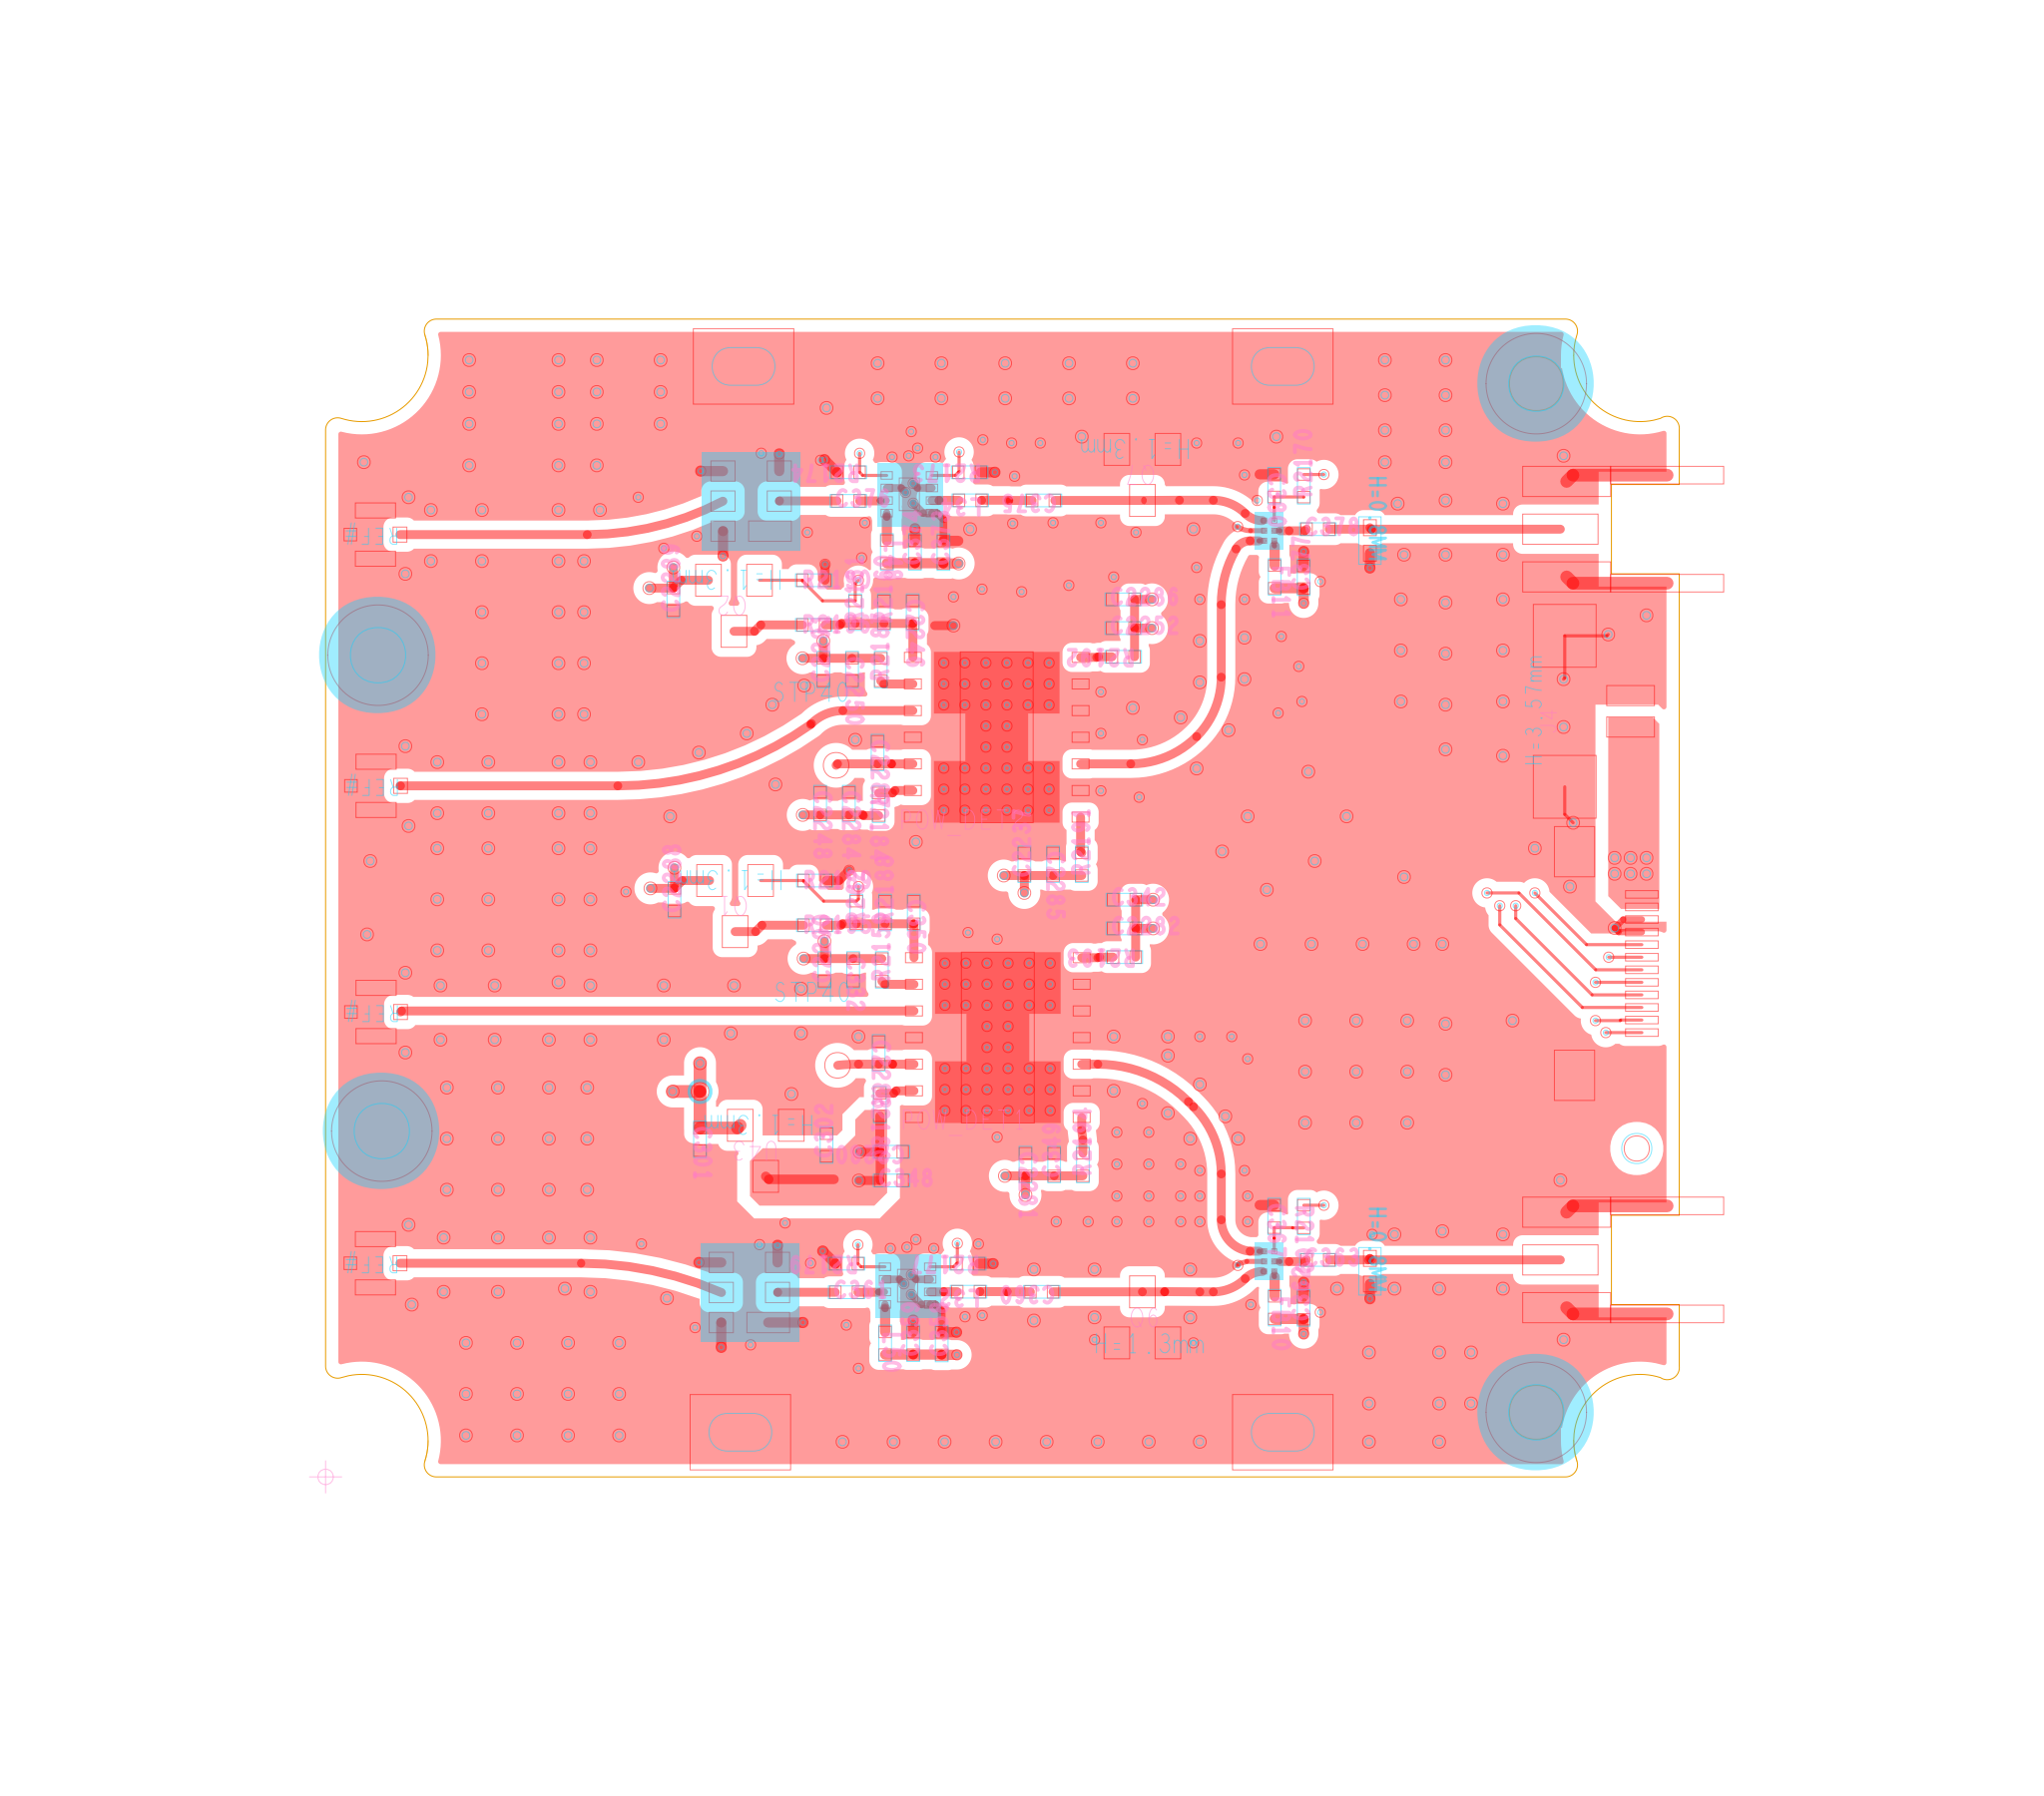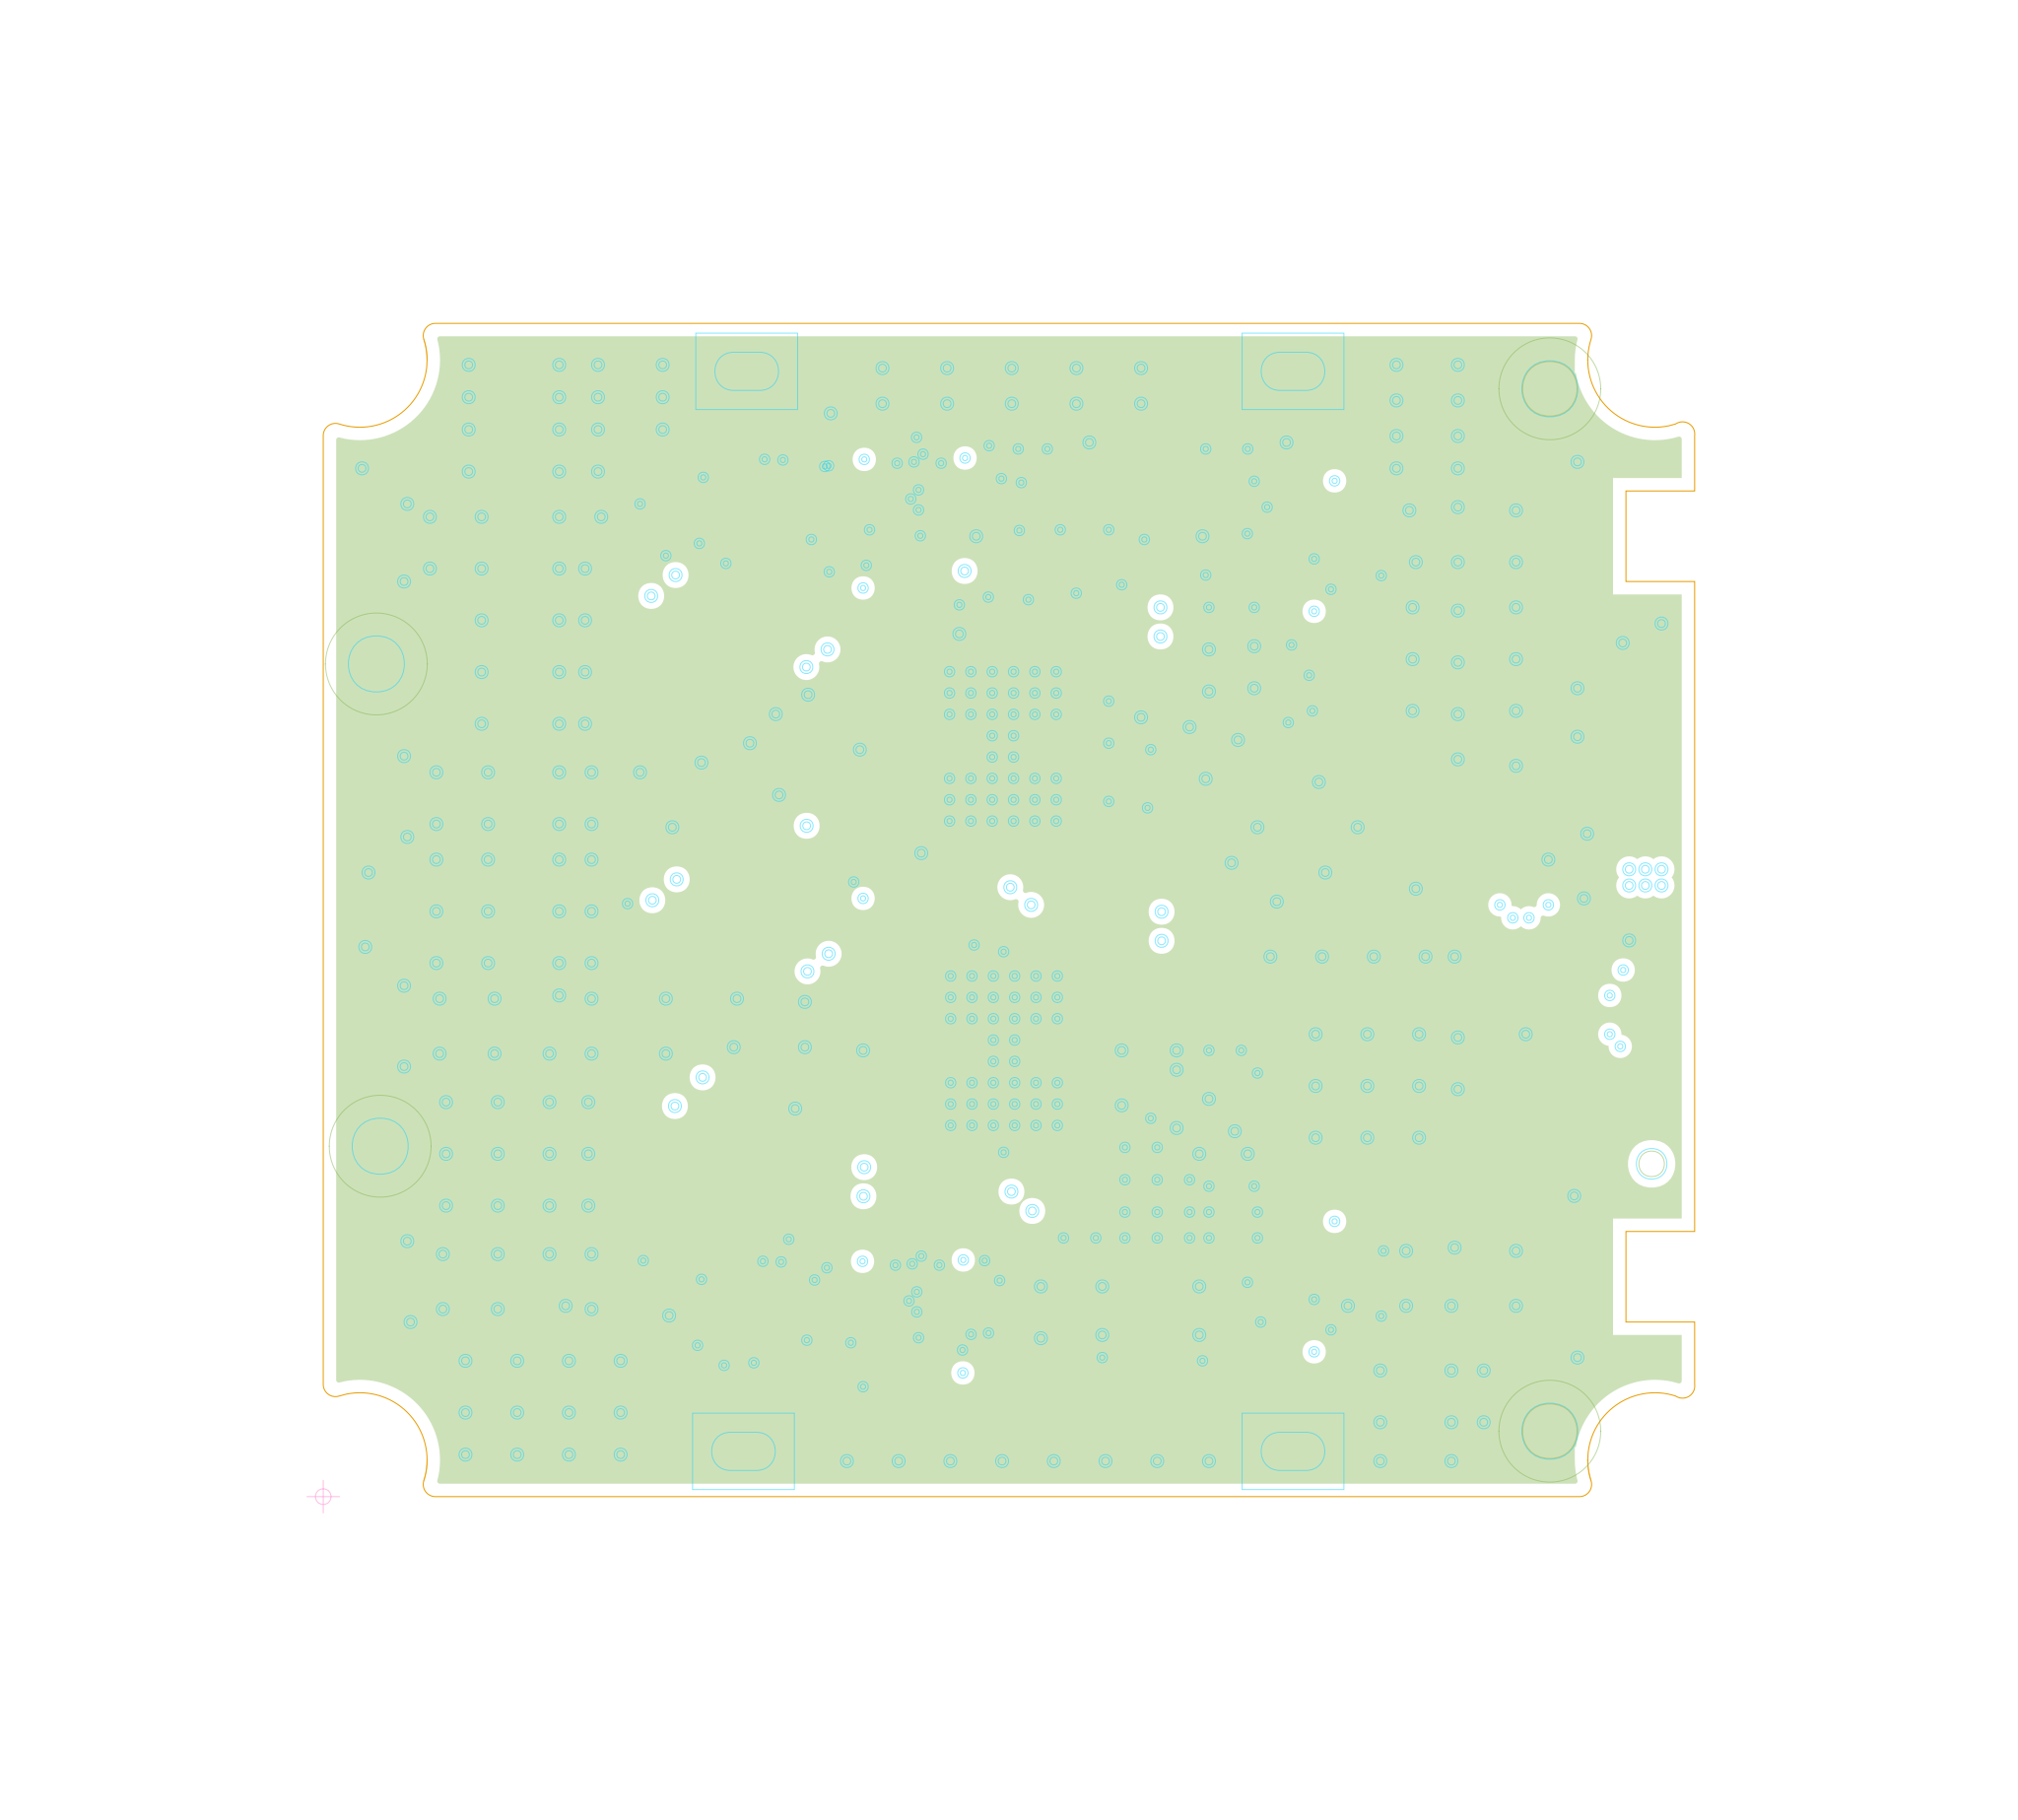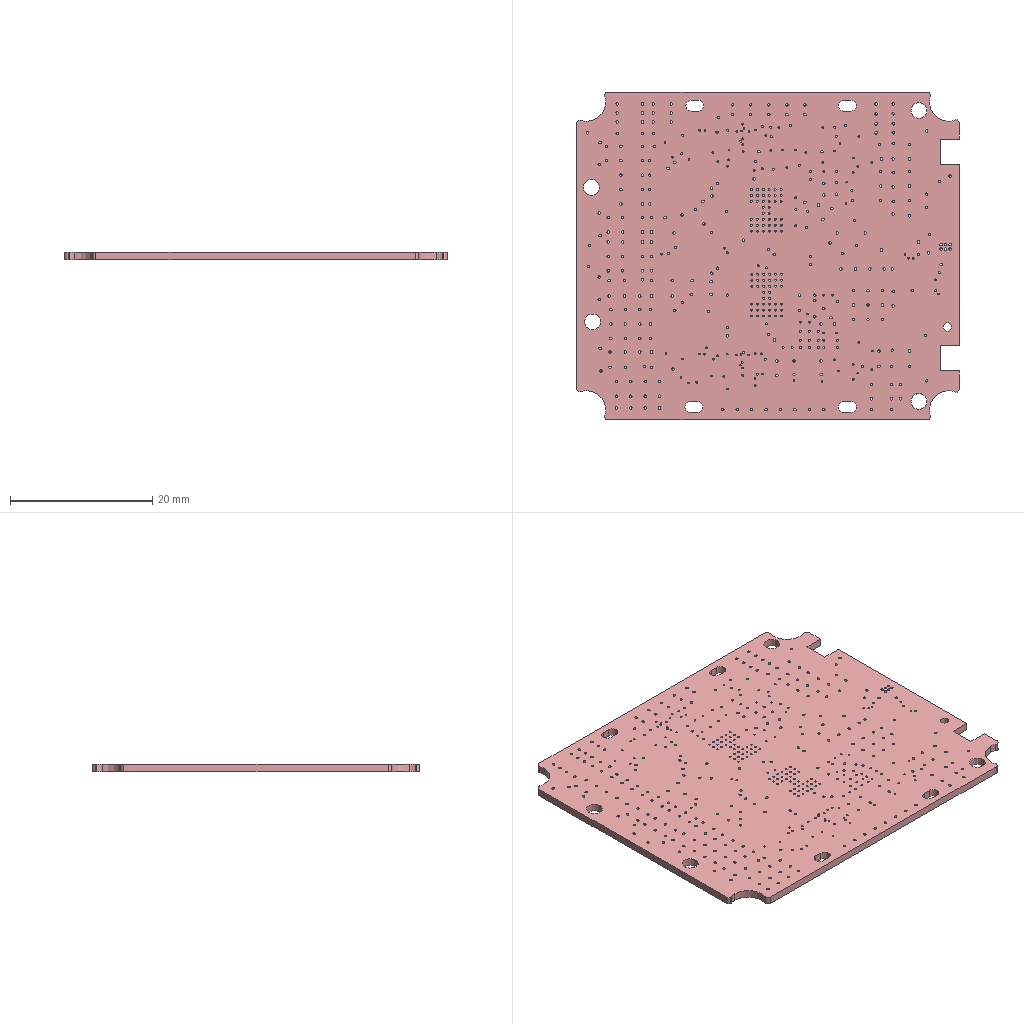Circuit board layout | Cadence Allegro | box 53.9 x 46.1 x 1.1 mm
Layer stack:
# Cadence Allegro layer stack of  (unit mm; from the constraint file cross-section; dielectric type: 0 not recorded (Allegro does not mark core vs prepreg), 3 surface material)
index,name,kind,layer,copper_thickness_mm,dielectric_type,dielectric_thickness_mm,dielectric_material,dielectric_constant
0,Top Surface,other,,,,,,
1,TOP,copper,TOP,0.0483,,,,
2,Dielectric1,dielectric,,,0,0.2032,FR-4,4.5
3,GND2,copper,GND2,0.0305,,,,
4,Dielectric2,dielectric,,,0,0.635,FR-4,4.5
5,POWER3,copper,POWER3,0.0305,,,,
6,Dielectric3,dielectric,,,0,0.2032,FR-4,4.5
7,BOTTOM,copper,BOTTOM,0.0483,,,,
8,Bottom Surface,other,,,,,,
# drill layer pairs: low layer,high layer
drill_pair,TOP,BOTTOM
Part placement:
REFDES,COMP_VALUE,SYM_NAME,SYM_X,SYM_Y,SYM_ROTATE,SYM_MIRROR
BM2,PESD0402V05,TVS0402,1636.51,322.35,270.000,NO
BM3,PESD0402V05,TVS0402,1636.51,1467.35,270.000,NO
C301,1uF,C0402_D,586.74,528.95,270.000,NO
C302,1uF,C0402_D,785.00,520.00,90.000,NO
C332,4.7uF,C0402_D,826.74,794.43,270.000,NO
C342,4.7uF,C0402_D,1251.74,904.43,0.000,NO
C348,4.7uF,C0402_D,886.74,464.43,0.000,NO
C349,4.7uF,C0402_D,1141.74,489.43,90.000,NO
C350,100pF,C0402_D,921.74,884.43,270.000,NO
C358,1nF,C0402_D,965.50,209.00,90.000,NO
C359,1uF,C0402_D,920.84,209.39,90.000,NO
C360,1nF,C0402_D,1122.28,290.00,180.000,NO
C361,1nF,C0402_D,816.48,289.32,0.000,NO
C362,1nF,C0402_D,1532.73,264.74,90.000,NO
C363,47pF,C0402_D,1555.00,340.00,0.000,NO
C367,47pF,C0402_D,1486.56,408.22,270.000,NO
C373,1nF,C0402_D,968.21,1449.00,90.000,NO
C374,1uF,C0402_D,923.55,1449.39,90.000,NO
C375,1nF,C0402_D,1124.99,1530.00,180.000,NO
C376,1nF,C0402_D,819.19,1529.32,0.000,NO
C377,1nF,C0402_D,1532.73,1409.74,90.000,NO
C378,47pF,C0402_D,1555.00,1485.00,0.000,NO
C380,47pF,C0402_D,1486.56,1553.22,270.000,NO
C2237,4.7uF,C0402_D,1095.00,960.00,90.000,NO
C2246,100pF,C0402_D,920.00,1355.00,270.000,NO
C2248,4.7uF,C0402_D,775.00,1055.00,270.000,NO
C2250,4.7uF,C0402_D,825.00,1265.00,270.000,NO
C2252,4.7uF,C0402_D,1250.00,1330.00,0.000,NO
C2280,100pF,C0402_D,886.74,509.43,180.000,NO
C2281,100pF,C0402_D,1096.74,489.43,270.000,NO
C2282,100pF,C0402_D,1251.74,859.43,0.000,NO
C2283,2.2nF,C0402_D,866.74,664.43,270.000,NO
C2284,100pF,C0402_D,820.00,1055.00,270.000,NO
C2285,100pF,C0402_D,1140.00,960.00,270.000,NO
C2286,100pF,C0402_D,1250.00,1375.00,0.000,NO
C2287,2.2nF,C0402_D,865.00,1135.00,270.000,NO
C2288,100nF,C0402_D,546.74,904.43,90.000,NO
C2289,100nF,C0402_D,545.00,1375.00,90.000,NO
C2290,100pF,C0402_D,781.74,794.43,90.000,NO
C2291,100pF,C0402_D,780.00,1265.00,90.000,NO
FB10,BLM15PD121SN1,L0402_D,1487.25,265.23,270.000,NO
FB11,BLM15PD121SN1,L0402_D,1487.25,1410.23,270.000,NO
J4,B2S,CNTR-2-1_25-A1251WRS,2045.00,1199.61,90.000,NO
J23,MMCX,MMCX008-H,1935.00,340.00,180.000,NO
J26,MMCX,MMCX008-H,1935.00,1485.00,180.000,NO
J32,HEADER 12,FPC_0_5_12PIN,2009.92,804.46,270.000,NO
L32,2.7nH,L0402_D,1007.55,290.17,180.000,NO
L34,2.7nH,L0402_D,1010.26,1530.17,180.000,NO
L48,47nH,L0402_D,879.56,1449.41,270.000,NO
L50,47nH,L0402_D,876.85,209.41,270.000,NO
POW_DET1,T POINT F,STP40,802.24,644.93,0.000,NO
POW_DET2,T POINT F,STP40,800.00,1115.00,0.000,NO
Q1,BM3139KT/DNP,SOT-23,641.74,894.43,180.000,NO
Q2,BM3139KT/DNP,SOT-23,640.00,1365.00,180.000,NO
Q6,SMP1330-005LF,SOT-23,1280.00,250.00,0.000,NO
Q7,SMP1330-005LF,SOT-23,1280.00,1570.00,180.000,NO
R262,0R,R0402_D,831.74,884.43,90.000,NO
R2159,0R,R0402_D,871.74,794.43,90.000,NO
R2160,10K,R0402_D,875.00,1355.00,90.000,NO
R2161,0R,R0402_D,830.00,1355.00,90.000,NO
R2169,22R,R0402_D,1532.92,407.92,270.000,NO
R2170,22R,R0402_D,1532.92,1552.92,90.000,NO
R2173,10K,R0402_D,1009.26,1574.13,180.000,NO
R2174,10K,R0402_D,819.14,1574.13,180.000,NO
R2177,10K,R0402_D,1006.55,334.13,180.000,NO
R2179,10K,R0402_D,816.43,334.13,180.000,NO
R2180,0R,R0402_D,868.48,583.38,270.000,NO
R2184,0R,R0402_D,866.74,1053.95,270.000,NO
R2187,0R,R0402_D,870.00,1265.00,90.000,NO
R2188,10K,R0402_D,876.74,884.43,90.000,NO
R2189,10K,R0402_D,766.74,934.43,0.000,NO
R2190,10K,R0402_D,765.00,1405.00,0.000,NO
R2191,0R,R0402_D,1185.00,960.00,90.000,NO
R2192,0R,R0402_D,1250.00,1285.00,180.000,NO
R2193,0R,R0402_D,1251.74,814.43,180.000,NO
R2194,0R,R0402_D,1186.74,489.43,90.000,NO
R2195,0R,R0402_D,766.74,864.43,0.000,NO
R2196,0R,R0402_D,765.00,1335.00,0.000,NO
SCR4,SCR,HOLE2_2_4,88.08,541.86,0.000,NO
SCR5,SCR,HOLE2_2_4,82.17,1287.53,0.000,NO
SCR6,SCR,HOLE2_2_4,1897.25,1712.99,0.000,NO
SCR7,SCR,HOLE2_2_4,1897.25,101.18,0.000,NO
U43,RT9166-33GVL,SOT-23,689.74,510.95,180.000,NO
U44,ZD9098,DFN2X2-8P,912.03,299.71,180.000,NO
U46,LX8625EH,DFN6_1_1_0_7MM,1478.74,337.65,180.000,NO
U49,ZD9098,DFN2X2-8P,914.74,1539.71,180.000,NO
U51,LX8625EH,DFN6_1_1_0_7MM,1478.74,1482.65,180.000,NO
U61,GCM1437A,PA-14-1_06-GCM1437A,1053.48,688.38,0.000,NO
U63,GCM1437A,PA-14-1_06-GCM1437A,1051.74,1158.95,0.000,NO
U65,TA2485A,TA2494A,664.16,288.96,180.000,NO
U66,TA2485A,TA2494A,666.87,1528.96,180.000,NO
U93,IPEX4-TXZ+214,IPEX4-2,79.11,728.47,180.000,NO
U94,IPEX4-TXZ+214,IPEX4-2,79.12,1082.80,180.000,NO
U95,IPEX4-TXZ+214,IPEX4-2,78.15,334.77,180.000,NO
U96,IPEX4-TXZ+214,IPEX4-2,78.15,1476.50,180.000,NO
VDD_3V3_RF,LABTESTPOINT,LTPT28C49P,586.74,603.95,180.000,NO
Pad and via stacks, first 110 of 129 lines:
# Allegro (Cadence) via spans and padstacks; design units: ("mils" 2 100)
# via spans: padstack,start_layer,end_layer,net_example,count
R3_0X4_0DO1_5X2_5,ETCH/TOP,ETCH/BOTTOM,GND,4
VIA_12_20,ETCH/TOP,ETCH/BOTTOM,GND,271
VIA8-16,ETCH/TOP,ETCH/BOTTOM,GND,217
# Allegro padstack definitions: name,start_layer,end_layer,drill,plating,holeType,type
TPT28C49P,"ETCH/TOP","ETCH/TOP",0.0,"PLATED","none","smd"
SMD25_20,"ETCH/TOP","ETCH/TOP",0.0,"PLATED","none","smd"
R0_455X0_5,"ETCH/TOP","ETCH/TOP",0.0,"PLATED","none","smd"
R1_5X1_3,"ETCH/TOP","ETCH/TOP",0.0,"PLATED","none","smd"
SMD22_20-A,"ETCH/TOP","ETCH/TOP",0.0,"PLATED","none","smd"
R1_4X2_6,"ETCH/TOP","ETCH/TOP",0.0,"PLATED","none","smd"
R0_9X0_9,"ETCH/TOP","ETCH/TOP",0.0,"PLATED","none","smd"
R0_7X0_5,"ETCH/TOP","ETCH/TOP",0.0,"PLATED","none","smd"
SMD1R20X1R60,"ETCH/TOP","ETCH/TOP",0.0,"PLATED","none","smd"
SMD3R00X1R50,"ETCH/TOP","ETCH/TOP",0.0,"PLATED","none","smd"
SMD100_180,"ETCH/TOP","ETCH/TOP",0.0,"PLATED","none","smd"
R032X024S,"ETCH/TOP","ETCH/TOP",0.0,"PLATED","none","smd"
SMD25_40,"ETCH/TOP","ETCH/TOP",0.0,"PLATED","none","smd"
SMD52_52,"ETCH/TOP","ETCH/TOP",0.0,"PLATED","none","smd"
BALL40,"ETCH/TOP","ETCH/TOP",0.0,"PLATED","none","smd"
R1_65X1_6,"ETCH/TOP","ETCH/TOP",0.0,"PLATED","none","smd"
R1_0X1_5,"ETCH/TOP","ETCH/TOP",0.0,"PLATED","none","smd"
REC87X31,"ETCH/TOP","ETCH/TOP",0.0,"PLATED","none","smd"
SMD67_224,"ETCH/TOP","ETCH/TOP",0.0,"PLATED","none","smd"
SMD165_165,"ETCH/TOP","ETCH/TOP",0.0,"PLATED","none","smd"
S_R3R40X1R30,"ETCH/TOP","ETCH/TOP",0.0,"PLATED","none","smd"
SMD50_30,"ETCH/TOP","ETCH/TOP",0.0,"PLATED","none","smd"
R1_02X1_27,"ETCH/TOP","ETCH/TOP",0.0,"PLATED","none","smd"
R2_5X1_7,"ETCH/TOP","ETCH/TOP",0.0,"PLATED","none","smd"
SMD30_50,"ETCH/TOP","ETCH/TOP",0.0,"PLATED","none","smd"
SMD25_50,"ETCH/TOP","ETCH/TOP",0.0,"PLATED","none","smd"
O025X075S,"ETCH/TOP","ETCH/TOP",0.0,"PLATED","none","smd"
O0_675X1_2,"ETCH/TOP","ETCH/TOP",0.0,"PLATED","none","smd"
O0_45X1_2,"ETCH/TOP","ETCH/TOP",0.0,"PLATED","none","smd"
SMD14_60,"ETCH/TOP","ETCH/TOP",0.0,"PLATED","none","smd"
REC75X25,"ETCH/TOP","ETCH/TOP",0.0,"PLATED","none","smd"
SMD10_60-S4,"ETCH/TOP","ETCH/TOP",0.0,"PLATED","none","smd"
SMD0R76X1R90,"ETCH/TOP","ETCH/TOP",0.0,"PLATED","none","smd"
S_S3R50,"ETCH/TOP","ETCH/TOP",0.0,"PLATED","none","smd"
S_R0R25X0R65,"ETCH/TOP","ETCH/TOP",0.0,"PLATED","none","smd"
S_R0R65X0R25,"ETCH/TOP","ETCH/TOP",0.0,"PLATED","none","smd"
SMD128_106,"ETCH/TOP","ETCH/TOP",0.0,"PLATED","none","smd"
SMD25_70,"ETCH/TOP","ETCH/TOP",0.0,"PLATED","none","smd"
C0_4X0_4,"ETCH/TOP","ETCH/TOP",0.0,"PLATED","none","smd"
R0_25X0_5,"ETCH/TOP","ETCH/TOP",0.0,"PLATED","none","smd"
R1_6X1_6PS0,"ETCH/TOP","ETCH/TOP",0.0,"PLATED","none","smd"
C0_25X0_25,"ETCH/TOP","ETCH/TOP",0.0,"PLATED","none","smd"
R1_0X1_0,"ETCH/TOP","ETCH/TOP",0.0,"PLATED","none","smd"
R0_2X0_4,"ETCH/TOP","ETCH/TOP",0.0,"PLATED","none","smd"
VQFN14-P-NP,"ETCH/TOP","ETCH/TOP",0.0,"PLATED","none","smd"
SMD32_10OB-S4,"ETCH/TOP","ETCH/TOP",0.0,"PLATED","none","smd"
SMD10_32OB-S4,"ETCH/TOP","ETCH/TOP",0.0,"PLATED","none","smd"
R015X032S,"ETCH/TOP","ETCH/TOP",0.0,"PLATED","none","smd"
SMD65_47,"ETCH/TOP","ETCH/TOP",0.0,"PLATED","none","smd"
SR100_125,"ETCH/TOP","ETCH/TOP",0.0,"PLATED","none","smd"
S_R1R40X1R20,"ETCH/TOP","ETCH/TOP",0.0,"NON_PLATED","none","smd"
SMD63_31D5,"ETCH/TOP","ETCH/TOP",0.0,"PLATED","none","smd"
S_C0R30,"ETCH/TOP","ETCH/TOP",0.0,"PLATED","none","smd"
SMD12_48,"ETCH/TOP","ETCH/TOP",0.0,"PLATED","none","smd"
S32,"ETCH/TOP","ETCH/TOP",0.0,"PLATED","none","smd"
R3_6X3_6PS0,"ETCH/TOP","ETCH/TOP",0.0,"PLATED","none","smd"
R0_25X0_7,"ETCH/TOP","ETCH/TOP",0.0,"PLATED","none","smd"
1X2,"ETCH/TOP","ETCH/TOP",0.0,"PLATED","none","smd"
SMD197_63,"ETCH/TOP","ETCH/TOP",0.0,"PLATED","none","smd"
SMDB197_63,"ETCH/BOTTOM","ETCH/BOTTOM",0.0,"PLATED","none","smd"
R0_76X1_52,"ETCH/TOP","ETCH/TOP",0.0,"PLATED","none","smd"
R1_2X2_0,"ETCH/TOP","ETCH/TOP",0.0,"PLATED","none","smd"
R0_6X0_8,"ETCH/TOP","ETCH/TOP",0.0,"PLATED","none","smd"
R29_92X50,"ETCH/TOP","ETCH/TOP",0.0,"PLATED","none","smd"
SMD2R20X3R50,"ETCH/TOP","ETCH/TOP",0.0,"PLATED","none","smd"
REC10X34,"ETCH/TOP","ETCH/TOP",0.0,"PLATED","none","smd"
REC34X10,"ETCH/TOP","ETCH/TOP",0.0,"PLATED","none","smd"
REC11X33-SH,"ETCH/TOP","ETCH/TOP",0.0,"PLATED","none","smd"
VIA12_STD-TH,"ETCH/TOP","ETCH/TOP",12.0,"PLATED","circle_drill","smd"
C20,"ETCH/TOP","ETCH/TOP",0.0,"PLATED","none","smd"
C16,"ETCH/TOP","ETCH/TOP",0.0,"PLATED","none","smd"
SMD_0P4X0P5,"ETCH/TOP","ETCH/TOP",0.0,"PLATED","none","smd"
S17,"ETCH/TOP","ETCH/TOP",0.0,"PLATED","none","smd"
SMD_R1933X850P0S20,"ETCH/TOP","ETCH/TOP",0.0,"PLATED","none","smd"
SMD_R2799X890P0S20,"ETCH/TOP","ETCH/TOP",0.0,"PLATED","none","smd"
SMD_R177X118P0S20,"ETCH/TOP","ETCH/TOP",0.0,"PLATED","none","smd"
SMD_R315X512P0S20,"ETCH/TOP","ETCH/TOP",0.0,"PLATED","none","smd"
SMD_RR79X79R50S20,"ETCH/TOP","ETCH/TOP",0.0,"PLATED","none","smd"
R96_81,"ETCH/TOP","ETCH/TOP",0.0,"PLATED","none","smd"
R170_81,"ETCH/TOP","ETCH/TOP",0.0,"PLATED","none","smd"
R100_35,"ETCH/TOP","ETCH/TOP",0.0,"PLATED","none","smd"
SMD_R118X512P0S20,"ETCH/TOP","ETCH/TOP",0.0,"PLATED","none","smd"
SMD_R787X630P0S20,"ETCH/TOP","ETCH/TOP",0.0,"PLATED","none","smd"
RECTX1_0Y1_05_IPEX1_ANTENNA,"ETCH/TOP","ETCH/TOP",0.0,"PLATED","none","smd"
RECTX1_05Y2_2_IPEX1_GROUND,"ETCH/TOP","ETCH/TOP",0.0,"PLATED","none","smd"
R4_0X2_0DR3_0X1_0,"ETCH/TOP","ETCH/BOTTOM",39.37,"PLATED","rectangle slot","through"
R4_5X2_0DR3_5X1_0,"ETCH/TOP","ETCH/BOTTOM",39.37,"PLATED","rectangle slot","through"
R2_0X4_0DR1_0X3_0,"ETCH/TOP","ETCH/BOTTOM",39.37,"PLATED","rectangle slot","through"
THC1R50D1R00,"ETCH/TOP","ETCH/BOTTOM",39.37,"PLATED","circle_drill","through"
THS1R50D1R00,"ETCH/TOP","ETCH/BOTTOM",39.37,"PLATED","circle_drill","through"
TH1_4C0_9,"ETCH/TOP","ETCH/BOTTOM",35.43,"PLATED","circle_drill","through"
TH3C1_8,"ETCH/TOP","ETCH/BOTTOM",70.87,"PLATED","circle_drill","through"
TH3_25C,"ETCH/TOP","ETCH/BOTTOM",127.95,"PLATED","circle_drill","through"
PAD240CIR118D,"ETCH/TOP","ETCH/BOTTOM",118.0,"PLATED","circle_drill","through"
VIA,"ETCH/TOP","ETCH/BOTTOM",13.0,"PLATED","circle_drill","through"
PAD118CIR88D-F,"ETCH/TOP","ETCH/BOTTOM",88.0,"PLATED","circle_drill","through"
PAD56CIR36D-F,"ETCH/TOP","ETCH/BOTTOM",36.0,"PLATED","circle_drill","through"
VIA0_5H0_3,"ETCH/TOP","ETCH/BOTTOM",11.81,"PLATED","circle_drill","through"
HOLE2_2_4,"ETCH/TOP","ETCH/BOTTOM",86.61,"PLATED","circle_drill","through"
VIA_12_20,"ETCH/TOP","ETCH/BOTTOM",12.0,"PLATED","circle_drill","through"
VIA8-16,"ETCH/TOP","ETCH/BOTTOM",8.0,"PLATED","circle_drill","through"
C4_0X4_0DC3_3,"ETCH/TOP","ETCH/BOTTOM",129.92,"PLATED","circle_drill","through"
F152,"ETCH/TOP","ETCH/BOTTOM",40.0,"PLATED","circle_drill","through"
F15,"ETCH/TOP","ETCH/BOTTOM",40.0,"PLATED","circle_drill","through"
Design rules, without the lines most boards share, first 18 of 43 lines:
# Cadence Allegro design rules of  (from the Constraint Manager export constraints.dcfx, design unit mil; typed fields in mm)
# columns: name | kind | enabled | priority | scope1 | scope2 | descriptor | typed fields (field=value)
# Allegro precedence (priority 1 wins): 1 Region class-to-class, 2 Region class, 3 Region, 4 class-to-class, 5 DiffPair/Bus/NetGroup override, 6 NetClass, 7 constraint set (CSet) default
# per-layer values are written LAYER=value in the descriptor and LAYER:mm in the typed field; a maximum of 0 means no limit set
# --- net classes (and buses / net groups) ---
9361_SPI | NetClass | enabled | 6 | no members | All | Net Class (members: 0) |
LVDS1 | NetClass | enabled | 6 | no members | All | Net Class (members: 0) |
LVDS0 | NetClass | enabled | 6 | no members | All | Net Class (members: 0) |
USB | NetClass | enabled | 6 | no members | All | Net Class (members: 0) |
PHY0_TX | NetClass | enabled | 6 | no members | All | Net Class (members: 0) |
PHY0_RX | NetClass | enabled | 6 | no members | All | Net Class (members: 0) |
PHY1_TX | NetClass | enabled | 6 | no members | All | Net Class (members: 0) |
PHY1_RD | NetClass | enabled | 6 | no members | All | Net Class (members: 0) |
EMMC | NetClass | enabled | 6 | no members | All | Net Class (members: 0) |
QSPI | NetClass | enabled | 6 | no members | All | Net Class (members: 0) |
DDR3_A | NetClass | enabled | 6 | no members | All | Net Class (members: 0) |
DDR1_DH | NetClass | enabled | 6 | no members | All | Net Class (members: 0) |
DDR1_DL | NetClass | enabled | 6 | no members | All | Net Class (members: 0) |